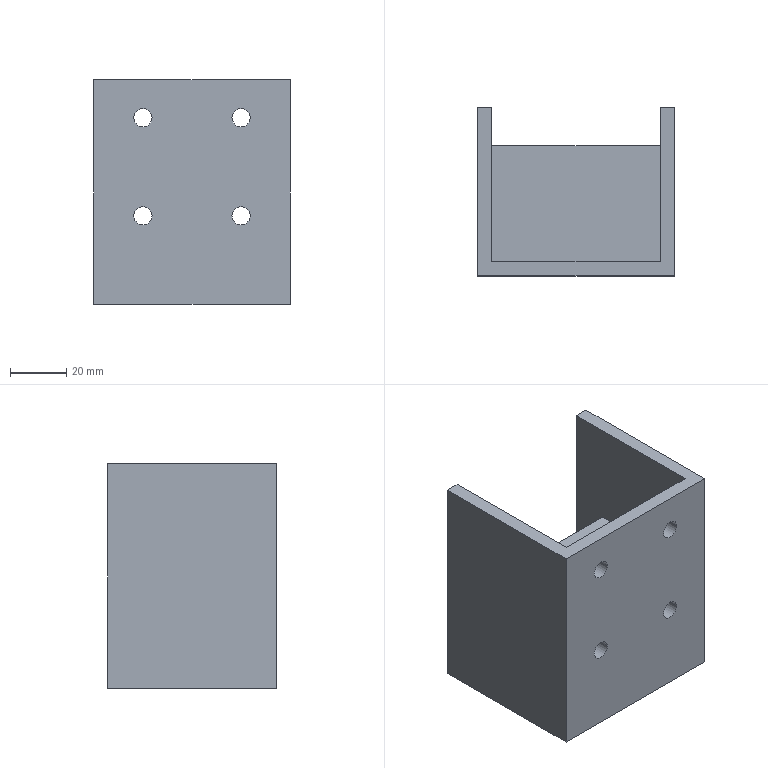Part | SolidWorks | features Cut 1, Extrusion 1, ICE 1 | 1 solid | 22 faces | box 70 x 60 x 80 mm | volume 83779 mm3 | plane 14 | cylinder 8 | commonest cylinder face diameters 6.5 x8
STEP:
#1=CARTESIAN_POINT('',(-20.75,-25.,26.5));
#2=VERTEX_POINT('',#1);
#3=CARTESIAN_POINT('',(-14.25,-25.,26.5));
#4=VERTEX_POINT('',#3);
#5=CARTESIAN_POINT('',(-17.5,-25.,26.5));
#6=DIRECTION('',(0.,-1.,0.));
#7=DIRECTION('',(0.,0.,-1.));
#8=AXIS2_PLACEMENT_3D('',#5,#6,#7);
#9=CIRCLE('',#8,3.25);
#10=EDGE_CURVE('',#2,#4,#9,.T.);
#11=ORIENTED_EDGE('',*,*,#10,.F.);
#12=CARTESIAN_POINT('',(-20.75,-30.,26.5));
#13=VERTEX_POINT('',#12);
#14=CARTESIAN_POINT('',(-20.75,-20.,26.5));
#15=DIRECTION('',(0.,-1.,0.));
#16=VECTOR('',#15,1000.);
#17=LINE('',#14,#16);
#18=EDGE_CURVE('',#2,#13,#17,.T.);
#19=ORIENTED_EDGE('',*,*,#18,.T.);
#20=CARTESIAN_POINT('',(-14.25,-30.,26.5));
#21=VERTEX_POINT('',#20);
#22=CARTESIAN_POINT('',(-17.5,-30.,26.5));
#23=DIRECTION('',(0.,-1.,0.));
#24=DIRECTION('',(1.,0.,0.));
#25=AXIS2_PLACEMENT_3D('',#22,#23,#24);
#26=CIRCLE('',#25,3.25);
#27=EDGE_CURVE('',#13,#21,#26,.T.);
#28=ORIENTED_EDGE('',*,*,#27,.T.);
#29=CARTESIAN_POINT('',(-14.25,-20.,26.5));
#30=DIRECTION('',(0.,-1.,0.));
#31=VECTOR('',#30,1000.);
#32=LINE('',#29,#31);
#33=EDGE_CURVE('',#4,#21,#32,.T.);
#34=ORIENTED_EDGE('',*,*,#33,.F.);
#35=EDGE_LOOP('',(#11,#19,#28,#34));
#36=FACE_OUTER_BOUND('',#35,.T.);
#37=CARTESIAN_POINT('',(-17.5,-20.,26.5));
#38=DIRECTION('',(0.,-1.,0.));
#39=DIRECTION('',(1.,0.,0.));
#40=AXIS2_PLACEMENT_3D('',#37,#38,#39);
#41=CYLINDRICAL_SURFACE('',#40,3.25);
#42=ADVANCED_FACE('',(#36),#41,.F.);
#43=CARTESIAN_POINT('',(-20.75,-25.,-8.5));
#44=VERTEX_POINT('',#43);
#45=CARTESIAN_POINT('',(-14.25,-25.,-8.5));
#46=VERTEX_POINT('',#45);
#47=CARTESIAN_POINT('',(-17.5,-25.,-8.5));
#48=DIRECTION('',(0.,-1.,0.));
#49=DIRECTION('',(0.,0.,-1.));
#50=AXIS2_PLACEMENT_3D('',#47,#48,#49);
#51=CIRCLE('',#50,3.25);
#52=EDGE_CURVE('',#44,#46,#51,.T.);
#53=ORIENTED_EDGE('',*,*,#52,.F.);
#54=CARTESIAN_POINT('',(-20.75,-30.,-8.5));
#55=VERTEX_POINT('',#54);
#56=CARTESIAN_POINT('',(-20.75,-20.,-8.5));
#57=DIRECTION('',(0.,-1.,0.));
#58=VECTOR('',#57,1000.);
#59=LINE('',#56,#58);
#60=EDGE_CURVE('',#44,#55,#59,.T.);
#61=ORIENTED_EDGE('',*,*,#60,.T.);
#62=CARTESIAN_POINT('',(-14.25,-30.,-8.5));
#63=VERTEX_POINT('',#62);
#64=CARTESIAN_POINT('',(-17.5,-30.,-8.5));
#65=DIRECTION('',(0.,-1.,0.));
#66=DIRECTION('',(1.,0.,0.));
#67=AXIS2_PLACEMENT_3D('',#64,#65,#66);
#68=CIRCLE('',#67,3.25);
#69=EDGE_CURVE('',#55,#63,#68,.T.);
#70=ORIENTED_EDGE('',*,*,#69,.T.);
#71=CARTESIAN_POINT('',(-14.25,-20.,-8.5));
#72=DIRECTION('',(0.,-1.,0.));
#73=VECTOR('',#72,1000.);
#74=LINE('',#71,#73);
#75=EDGE_CURVE('',#46,#63,#74,.T.);
#76=ORIENTED_EDGE('',*,*,#75,.F.);
#77=EDGE_LOOP('',(#53,#61,#70,#76));
#78=FACE_OUTER_BOUND('',#77,.T.);
#79=CARTESIAN_POINT('',(-17.5,-20.,-8.5));
#80=DIRECTION('',(0.,-1.,0.));
#81=DIRECTION('',(1.,0.,0.));
#82=AXIS2_PLACEMENT_3D('',#79,#80,#81);
#83=CYLINDRICAL_SURFACE('',#82,3.25);
#84=ADVANCED_FACE('',(#78),#83,.F.);
#85=CARTESIAN_POINT('',(14.25,-25.,-8.5));
#86=VERTEX_POINT('',#85);
#87=CARTESIAN_POINT('',(20.75,-25.,-8.5));
#88=VERTEX_POINT('',#87);
#89=CARTESIAN_POINT('',(17.5,-25.,-8.5));
#90=DIRECTION('',(0.,-1.,0.));
#91=DIRECTION('',(0.,0.,-1.));
#92=AXIS2_PLACEMENT_3D('',#89,#90,#91);
#93=CIRCLE('',#92,3.25);
#94=EDGE_CURVE('',#86,#88,#93,.T.);
#95=ORIENTED_EDGE('',*,*,#94,.F.);
#96=CARTESIAN_POINT('',(14.25,-30.,-8.5));
#97=VERTEX_POINT('',#96);
#98=CARTESIAN_POINT('',(14.25,-20.,-8.5));
#99=DIRECTION('',(0.,-1.,0.));
#100=VECTOR('',#99,1000.);
#101=LINE('',#98,#100);
#102=EDGE_CURVE('',#86,#97,#101,.T.);
#103=ORIENTED_EDGE('',*,*,#102,.T.);
#104=CARTESIAN_POINT('',(20.75,-30.,-8.5));
#105=VERTEX_POINT('',#104);
#106=CARTESIAN_POINT('',(17.5,-30.,-8.5));
#107=DIRECTION('',(0.,-1.,0.));
#108=DIRECTION('',(1.,0.,0.));
#109=AXIS2_PLACEMENT_3D('',#106,#107,#108);
#110=CIRCLE('',#109,3.25);
#111=EDGE_CURVE('',#97,#105,#110,.T.);
#112=ORIENTED_EDGE('',*,*,#111,.T.);
#113=CARTESIAN_POINT('',(20.75,-20.,-8.5));
#114=DIRECTION('',(0.,-1.,0.));
#115=VECTOR('',#114,1000.);
#116=LINE('',#113,#115);
#117=EDGE_CURVE('',#88,#105,#116,.T.);
#118=ORIENTED_EDGE('',*,*,#117,.F.);
#119=EDGE_LOOP('',(#95,#103,#112,#118));
#120=FACE_OUTER_BOUND('',#119,.T.);
#121=CARTESIAN_POINT('',(17.5,-20.,-8.5));
#122=DIRECTION('',(0.,-1.,0.));
#123=DIRECTION('',(1.,0.,0.));
#124=AXIS2_PLACEMENT_3D('',#121,#122,#123);
#125=CYLINDRICAL_SURFACE('',#124,3.25);
#126=ADVANCED_FACE('',(#120),#125,.F.);
#127=CARTESIAN_POINT('',(14.25,-25.,26.5));
#128=VERTEX_POINT('',#127);
#129=CARTESIAN_POINT('',(20.75,-25.,26.5));
#130=VERTEX_POINT('',#129);
#131=CARTESIAN_POINT('',(17.5,-25.,26.5));
#132=DIRECTION('',(0.,-1.,0.));
#133=DIRECTION('',(0.,0.,-1.));
#134=AXIS2_PLACEMENT_3D('',#131,#132,#133);
#135=CIRCLE('',#134,3.25);
#136=EDGE_CURVE('',#128,#130,#135,.T.);
#137=ORIENTED_EDGE('',*,*,#136,.F.);
#138=CARTESIAN_POINT('',(14.25,-30.,26.5));
#139=VERTEX_POINT('',#138);
#140=CARTESIAN_POINT('',(14.25,-20.,26.5));
#141=DIRECTION('',(0.,-1.,0.));
#142=VECTOR('',#141,1000.);
#143=LINE('',#140,#142);
#144=EDGE_CURVE('',#128,#139,#143,.T.);
#145=ORIENTED_EDGE('',*,*,#144,.T.);
#146=CARTESIAN_POINT('',(20.75,-30.,26.5));
#147=VERTEX_POINT('',#146);
#148=CARTESIAN_POINT('',(17.5,-30.,26.5));
#149=DIRECTION('',(0.,-1.,0.));
#150=DIRECTION('',(1.,0.,0.));
#151=AXIS2_PLACEMENT_3D('',#148,#149,#150);
#152=CIRCLE('',#151,3.25);
#153=EDGE_CURVE('',#139,#147,#152,.T.);
#154=ORIENTED_EDGE('',*,*,#153,.T.);
#155=CARTESIAN_POINT('',(20.75,-20.,26.5));
#156=DIRECTION('',(0.,-1.,0.));
#157=VECTOR('',#156,1000.);
#158=LINE('',#155,#157);
#159=EDGE_CURVE('',#130,#147,#158,.T.);
#160=ORIENTED_EDGE('',*,*,#159,.F.);
#161=EDGE_LOOP('',(#137,#145,#154,#160));
#162=FACE_OUTER_BOUND('',#161,.T.);
#163=CARTESIAN_POINT('',(17.5,-20.,26.5));
#164=DIRECTION('',(0.,-1.,0.));
#165=DIRECTION('',(1.,0.,0.));
#166=AXIS2_PLACEMENT_3D('',#163,#164,#165);
#167=CYLINDRICAL_SURFACE('',#166,3.25);
#168=ADVANCED_FACE('',(#162),#167,.F.);
#169=CARTESIAN_POINT('',(30.,-25.,2.5));
#170=VERTEX_POINT('',#169);
#171=CARTESIAN_POINT('',(30.,16.476,2.5));
#172=VERTEX_POINT('',#171);
#173=CARTESIAN_POINT('',(30.,-25.,2.5));
#174=DIRECTION('',(0.,1.,0.));
#175=VECTOR('',#174,1000.);
#176=LINE('',#173,#175);
#177=EDGE_CURVE('',#170,#172,#176,.T.);
#178=ORIENTED_EDGE('',*,*,#177,.F.);
#179=CARTESIAN_POINT('',(30.,-25.,40.));
#180=VERTEX_POINT('',#179);
#181=CARTESIAN_POINT('',(30.,-25.,40.));
#182=DIRECTION('',(0.,0.,-1.));
#183=VECTOR('',#182,1000.);
#184=LINE('',#181,#183);
#185=EDGE_CURVE('',#180,#170,#184,.T.);
#186=ORIENTED_EDGE('',*,*,#185,.F.);
#187=CARTESIAN_POINT('',(30.,30.,40.));
#188=VERTEX_POINT('',#187);
#189=CARTESIAN_POINT('',(30.,-25.,40.));
#190=DIRECTION('',(0.,-1.,0.));
#191=VECTOR('',#190,1000.);
#192=LINE('',#189,#191);
#193=EDGE_CURVE('',#188,#180,#192,.T.);
#194=ORIENTED_EDGE('',*,*,#193,.F.);
#195=CARTESIAN_POINT('',(30.,30.,-40.));
#196=VERTEX_POINT('',#195);
#197=CARTESIAN_POINT('',(30.,30.,40.));
#198=DIRECTION('',(0.,0.,-1.));
#199=VECTOR('',#198,1000.);
#200=LINE('',#197,#199);
#201=EDGE_CURVE('',#188,#196,#200,.T.);
#202=ORIENTED_EDGE('',*,*,#201,.T.);
#203=CARTESIAN_POINT('',(30.,-25.,-40.));
#204=VERTEX_POINT('',#203);
#205=CARTESIAN_POINT('',(30.,-25.,-40.));
#206=DIRECTION('',(0.,-1.,0.));
#207=VECTOR('',#206,1000.);
#208=LINE('',#205,#207);
#209=EDGE_CURVE('',#196,#204,#208,.T.);
#210=ORIENTED_EDGE('',*,*,#209,.T.);
#211=CARTESIAN_POINT('',(30.,-25.,-2.5));
#212=VERTEX_POINT('',#211);
#213=CARTESIAN_POINT('',(30.,-25.,40.));
#214=DIRECTION('',(0.,0.,-1.));
#215=VECTOR('',#214,1000.);
#216=LINE('',#213,#215);
#217=EDGE_CURVE('',#212,#204,#216,.T.);
#218=ORIENTED_EDGE('',*,*,#217,.F.);
#219=CARTESIAN_POINT('',(30.,16.476,-2.5));
#220=VERTEX_POINT('',#219);
#221=CARTESIAN_POINT('',(30.,-25.,-2.5));
#222=DIRECTION('',(0.,1.,0.));
#223=VECTOR('',#222,1000.);
#224=LINE('',#221,#223);
#225=EDGE_CURVE('',#212,#220,#224,.T.);
#226=ORIENTED_EDGE('',*,*,#225,.T.);
#227=CARTESIAN_POINT('',(30.,16.476,2.5));
#228=DIRECTION('',(0.,0.,-1.));
#229=VECTOR('',#228,1000.);
#230=LINE('',#227,#229);
#231=EDGE_CURVE('',#172,#220,#230,.T.);
#232=ORIENTED_EDGE('',*,*,#231,.F.);
#233=EDGE_LOOP('',(#178,#186,#194,#202,#210,#218,#226,#232));
#234=FACE_OUTER_BOUND('',#233,.T.);
#235=CARTESIAN_POINT('',(30.,-25.,40.));
#236=DIRECTION('',(1.,0.,0.));
#237=DIRECTION('',(0.,1.,0.));
#238=AXIS2_PLACEMENT_3D('',#235,#236,#237);
#239=PLANE('',#238);
#240=ADVANCED_FACE('',(#234),#239,.F.);
#241=CARTESIAN_POINT('',(-17.5,-25.,26.5));
#242=DIRECTION('',(0.,-1.,0.));
#243=DIRECTION('',(0.,0.,-1.));
#244=AXIS2_PLACEMENT_3D('',#241,#242,#243);
#245=CIRCLE('',#244,3.25);
#246=EDGE_CURVE('',#4,#2,#245,.T.);
#247=ORIENTED_EDGE('',*,*,#246,.T.);
#248=ORIENTED_EDGE('',*,*,#10,.T.);
#249=EDGE_LOOP('',(#247,#248));
#250=FACE_BOUND('',#249,.T.);
#251=CARTESIAN_POINT('',(17.5,-25.,26.5));
#252=DIRECTION('',(0.,-1.,0.));
#253=DIRECTION('',(0.,0.,-1.));
#254=AXIS2_PLACEMENT_3D('',#251,#252,#253);
#255=CIRCLE('',#254,3.25);
#256=EDGE_CURVE('',#130,#128,#255,.T.);
#257=ORIENTED_EDGE('',*,*,#256,.T.);
#258=ORIENTED_EDGE('',*,*,#136,.T.);
#259=EDGE_LOOP('',(#257,#258));
#260=FACE_BOUND('',#259,.T.);
#261=CARTESIAN_POINT('',(-30.,-25.,2.5));
#262=VERTEX_POINT('',#261);
#263=CARTESIAN_POINT('',(-30.,-25.,2.5));
#264=DIRECTION('',(1.,0.,0.));
#265=VECTOR('',#264,1000.);
#266=LINE('',#263,#265);
#267=EDGE_CURVE('',#262,#170,#266,.T.);
#268=ORIENTED_EDGE('',*,*,#267,.F.);
#269=CARTESIAN_POINT('',(-30.,-25.,40.));
#270=VERTEX_POINT('',#269);
#271=CARTESIAN_POINT('',(-30.,-25.,40.));
#272=DIRECTION('',(0.,0.,-1.));
#273=VECTOR('',#272,1000.);
#274=LINE('',#271,#273);
#275=EDGE_CURVE('',#270,#262,#274,.T.);
#276=ORIENTED_EDGE('',*,*,#275,.F.);
#277=CARTESIAN_POINT('',(-30.,-25.,40.));
#278=DIRECTION('',(-1.,0.,0.));
#279=VECTOR('',#278,1000.);
#280=LINE('',#277,#279);
#281=EDGE_CURVE('',#180,#270,#280,.T.);
#282=ORIENTED_EDGE('',*,*,#281,.F.);
#283=ORIENTED_EDGE('',*,*,#185,.T.);
#284=EDGE_LOOP('',(#268,#276,#282,#283));
#285=FACE_OUTER_BOUND('',#284,.T.);
#286=CARTESIAN_POINT('',(-30.,-25.,40.));
#287=DIRECTION('',(0.,-1.,0.));
#288=DIRECTION('',(0.,0.,-1.));
#289=AXIS2_PLACEMENT_3D('',#286,#287,#288);
#290=PLANE('',#289);
#291=ADVANCED_FACE('',(#250,#260,#285),#290,.F.);
#292=CARTESIAN_POINT('',(-30.,16.476,2.5));
#293=VERTEX_POINT('',#292);
#294=CARTESIAN_POINT('',(-30.,-25.,2.5));
#295=DIRECTION('',(0.,-1.,0.));
#296=VECTOR('',#295,1000.);
#297=LINE('',#294,#296);
#298=EDGE_CURVE('',#293,#262,#297,.T.);
#299=ORIENTED_EDGE('',*,*,#298,.F.);
#300=CARTESIAN_POINT('',(-30.,16.476,-2.5));
#301=VERTEX_POINT('',#300);
#302=CARTESIAN_POINT('',(-30.,16.476,2.5));
#303=DIRECTION('',(0.,0.,-1.));
#304=VECTOR('',#303,1000.);
#305=LINE('',#302,#304);
#306=EDGE_CURVE('',#293,#301,#305,.T.);
#307=ORIENTED_EDGE('',*,*,#306,.T.);
#308=CARTESIAN_POINT('',(-30.,-25.,-2.5));
#309=VERTEX_POINT('',#308);
#310=CARTESIAN_POINT('',(-30.,-25.,-2.5));
#311=DIRECTION('',(0.,-1.,0.));
#312=VECTOR('',#311,1000.);
#313=LINE('',#310,#312);
#314=EDGE_CURVE('',#301,#309,#313,.T.);
#315=ORIENTED_EDGE('',*,*,#314,.T.);
#316=CARTESIAN_POINT('',(-30.,-25.,-40.));
#317=VERTEX_POINT('',#316);
#318=CARTESIAN_POINT('',(-30.,-25.,40.));
#319=DIRECTION('',(0.,0.,-1.));
#320=VECTOR('',#319,1000.);
#321=LINE('',#318,#320);
#322=EDGE_CURVE('',#309,#317,#321,.T.);
#323=ORIENTED_EDGE('',*,*,#322,.T.);
#324=CARTESIAN_POINT('',(-30.,30.,-40.));
#325=VERTEX_POINT('',#324);
#326=CARTESIAN_POINT('',(-30.,30.,-40.));
#327=DIRECTION('',(0.,1.,0.));
#328=VECTOR('',#327,1000.);
#329=LINE('',#326,#328);
#330=EDGE_CURVE('',#317,#325,#329,.T.);
#331=ORIENTED_EDGE('',*,*,#330,.T.);
#332=CARTESIAN_POINT('',(-30.,30.,40.));
#333=VERTEX_POINT('',#332);
#334=CARTESIAN_POINT('',(-30.,30.,40.));
#335=DIRECTION('',(0.,0.,-1.));
#336=VECTOR('',#335,1000.);
#337=LINE('',#334,#336);
#338=EDGE_CURVE('',#333,#325,#337,.T.);
#339=ORIENTED_EDGE('',*,*,#338,.F.);
#340=CARTESIAN_POINT('',(-30.,30.,40.));
#341=DIRECTION('',(0.,1.,0.));
#342=VECTOR('',#341,1000.);
#343=LINE('',#340,#342);
#344=EDGE_CURVE('',#270,#333,#343,.T.);
#345=ORIENTED_EDGE('',*,*,#344,.F.);
#346=ORIENTED_EDGE('',*,*,#275,.T.);
#347=EDGE_LOOP('',(#299,#307,#315,#323,#331,#339,#345,#346));
#348=FACE_OUTER_BOUND('',#347,.T.);
#349=CARTESIAN_POINT('',(-30.,30.,40.));
#350=DIRECTION('',(-1.,0.,0.));
#351=DIRECTION('',(0.,-1.,0.));
#352=AXIS2_PLACEMENT_3D('',#349,#350,#351);
#353=PLANE('',#352);
#354=ADVANCED_FACE('',(#348),#353,.F.);
#355=CARTESIAN_POINT('',(-35.,30.,-40.));
#356=VERTEX_POINT('',#355);
#357=CARTESIAN_POINT('',(-30.,30.,-40.));
#358=DIRECTION('',(-1.,0.,0.));
#359=VECTOR('',#358,1000.);
#360=LINE('',#357,#359);
#361=EDGE_CURVE('',#325,#356,#360,.T.);
#362=ORIENTED_EDGE('',*,*,#361,.T.);
#363=CARTESIAN_POINT('',(-35.,30.,40.));
#364=VERTEX_POINT('',#363);
#365=CARTESIAN_POINT('',(-35.,30.,40.));
#366=DIRECTION('',(0.,0.,-1.));
#367=VECTOR('',#366,1000.);
#368=LINE('',#365,#367);
#369=EDGE_CURVE('',#364,#356,#368,.T.);
#370=ORIENTED_EDGE('',*,*,#369,.F.);
#371=CARTESIAN_POINT('',(-30.,30.,40.));
#372=DIRECTION('',(-1.,0.,0.));
#373=VECTOR('',#372,1000.);
#374=LINE('',#371,#373);
#375=EDGE_CURVE('',#333,#364,#374,.T.);
#376=ORIENTED_EDGE('',*,*,#375,.F.);
#377=ORIENTED_EDGE('',*,*,#338,.T.);
#378=EDGE_LOOP('',(#362,#370,#376,#377));
#379=FACE_OUTER_BOUND('',#378,.T.);
#380=CARTESIAN_POINT('',(-30.,30.,40.));
#381=DIRECTION('',(0.,-1.,0.));
#382=DIRECTION('',(0.,0.,-1.));
#383=AXIS2_PLACEMENT_3D('',#380,#381,#382);
#384=PLANE('',#383);
#385=ADVANCED_FACE('',(#379),#384,.F.);
#386=CARTESIAN_POINT('',(-35.,-30.,-40.));
#387=VERTEX_POINT('',#386);
#388=CARTESIAN_POINT('',(-35.,-30.,-40.));
#389=DIRECTION('',(0.,-1.,0.));
#390=VECTOR('',#389,1000.);
#391=LINE('',#388,#390);
#392=EDGE_CURVE('',#356,#387,#391,.T.);
#393=ORIENTED_EDGE('',*,*,#392,.T.);
#394=CARTESIAN_POINT('',(-35.,-30.,40.));
#395=VERTEX_POINT('',#394);
#396=CARTESIAN_POINT('',(-35.,-30.,40.));
#397=DIRECTION('',(0.,0.,-1.));
#398=VECTOR('',#397,1000.);
#399=LINE('',#396,#398);
#400=EDGE_CURVE('',#395,#387,#399,.T.);
#401=ORIENTED_EDGE('',*,*,#400,.F.);
#402=CARTESIAN_POINT('',(-35.,-30.,40.));
#403=DIRECTION('',(0.,-1.,0.));
#404=VECTOR('',#403,1000.);
#405=LINE('',#402,#404);
#406=EDGE_CURVE('',#364,#395,#405,.T.);
#407=ORIENTED_EDGE('',*,*,#406,.F.);
#408=ORIENTED_EDGE('',*,*,#369,.T.);
#409=EDGE_LOOP('',(#393,#401,#407,#408));
#410=FACE_OUTER_BOUND('',#409,.T.);
#411=CARTESIAN_POINT('',(-35.,-30.,40.));
#412=DIRECTION('',(1.,0.,0.));
#413=DIRECTION('',(0.,0.,-1.));
#414=AXIS2_PLACEMENT_3D('',#411,#412,#413);
#415=PLANE('',#414);
#416=ADVANCED_FACE('',(#410),#415,.F.);
#417=CARTESIAN_POINT('',(-17.5,-30.,26.5));
#418=DIRECTION('',(0.,-1.,0.));
#419=DIRECTION('',(1.,0.,0.));
#420=AXIS2_PLACEMENT_3D('',#417,#418,#419);
#421=CIRCLE('',#420,3.25);
#422=EDGE_CURVE('',#21,#13,#421,.T.);
#423=ORIENTED_EDGE('',*,*,#422,.F.);
#424=ORIENTED_EDGE('',*,*,#27,.F.);
#425=EDGE_LOOP('',(#423,#424));
#426=FACE_BOUND('',#425,.T.);
#427=CARTESIAN_POINT('',(-17.5,-30.,-8.5));
#428=DIRECTION('',(0.,-1.,0.));
#429=DIRECTION('',(1.,0.,0.));
#430=AXIS2_PLACEMENT_3D('',#427,#428,#429);
#431=CIRCLE('',#430,3.25);
#432=EDGE_CURVE('',#63,#55,#431,.T.);
#433=ORIENTED_EDGE('',*,*,#432,.F.);
#434=ORIENTED_EDGE('',*,*,#69,.F.);
#435=EDGE_LOOP('',(#433,#434));
#436=FACE_BOUND('',#435,.T.);
#437=CARTESIAN_POINT('',(17.5,-30.,-8.5));
#438=DIRECTION('',(0.,-1.,0.));
#439=DIRECTION('',(1.,0.,0.));
#440=AXIS2_PLACEMENT_3D('',#437,#438,#439);
#441=CIRCLE('',#440,3.25);
#442=EDGE_CURVE('',#105,#97,#441,.T.);
#443=ORIENTED_EDGE('',*,*,#442,.F.);
#444=ORIENTED_EDGE('',*,*,#111,.F.);
#445=EDGE_LOOP('',(#443,#444));
#446=FACE_BOUND('',#445,.T.);
#447=CARTESIAN_POINT('',(17.5,-30.,26.5));
#448=DIRECTION('',(0.,-1.,0.));
#449=DIRECTION('',(1.,0.,0.));
#450=AXIS2_PLACEMENT_3D('',#447,#448,#449);
#451=CIRCLE('',#450,3.25);
#452=EDGE_CURVE('',#147,#139,#451,.T.);
#453=ORIENTED_EDGE('',*,*,#452,.F.);
#454=ORIENTED_EDGE('',*,*,#153,.F.);
#455=EDGE_LOOP('',(#453,#454));
#456=FACE_BOUND('',#455,.T.);
#457=CARTESIAN_POINT('',(35.,-30.,-40.));
#458=VERTEX_POINT('',#457);
#459=CARTESIAN_POINT('',(35.,-30.,-40.));
#460=DIRECTION('',(1.,0.,0.));
#461=VECTOR('',#460,1000.);
#462=LINE('',#459,#461);
#463=EDGE_CURVE('',#387,#458,#462,.T.);
#464=ORIENTED_EDGE('',*,*,#463,.T.);
#465=CARTESIAN_POINT('',(35.,-30.,40.));
#466=VERTEX_POINT('',#465);
#467=CARTESIAN_POINT('',(35.,-30.,40.));
#468=DIRECTION('',(0.,0.,-1.));
#469=VECTOR('',#468,1000.);
#470=LINE('',#467,#469);
#471=EDGE_CURVE('',#466,#458,#470,.T.);
#472=ORIENTED_EDGE('',*,*,#471,.F.);
#473=CARTESIAN_POINT('',(35.,-30.,40.));
#474=DIRECTION('',(1.,0.,0.));
#475=VECTOR('',#474,1000.);
#476=LINE('',#473,#475);
#477=EDGE_CURVE('',#395,#466,#476,.T.);
#478=ORIENTED_EDGE('',*,*,#477,.F.);
#479=ORIENTED_EDGE('',*,*,#400,.T.);
#480=EDGE_LOOP('',(#464,#472,#478,#479));
#481=FACE_OUTER_BOUND('',#480,.T.);
#482=CARTESIAN_POINT('',(35.,-30.,40.));
#483=DIRECTION('',(0.,1.,0.));
#484=DIRECTION('',(-1.,0.,0.));
#485=AXIS2_PLACEMENT_3D('',#482,#483,#484);
#486=PLANE('',#485);
#487=ADVANCED_FACE('',(#426,#436,#446,#456,#481),#486,.F.);
#488=CARTESIAN_POINT('',(35.,30.,-40.));
#489=VERTEX_POINT('',#488);
#490=CARTESIAN_POINT('',(35.,-30.,-40.));
#491=DIRECTION('',(0.,1.,0.));
#492=VECTOR('',#491,1000.);
#493=LINE('',#490,#492);
#494=EDGE_CURVE('',#458,#489,#493,.T.);
#495=ORIENTED_EDGE('',*,*,#494,.T.);
#496=CARTESIAN_POINT('',(35.,30.,40.));
#497=VERTEX_POINT('',#496);
#498=CARTESIAN_POINT('',(35.,30.,40.));
#499=DIRECTION('',(0.,0.,-1.));
#500=VECTOR('',#499,1000.);
#501=LINE('',#498,#500);
#502=EDGE_CURVE('',#497,#489,#501,.T.);
#503=ORIENTED_EDGE('',*,*,#502,.F.);
#504=CARTESIAN_POINT('',(35.,-30.,40.));
#505=DIRECTION('',(0.,1.,0.));
#506=VECTOR('',#505,1000.);
#507=LINE('',#504,#506);
#508=EDGE_CURVE('',#466,#497,#507,.T.);
#509=ORIENTED_EDGE('',*,*,#508,.F.);
#510=ORIENTED_EDGE('',*,*,#471,.T.);
#511=EDGE_LOOP('',(#495,#503,#509,#510));
#512=FACE_OUTER_BOUND('',#511,.T.);
#513=CARTESIAN_POINT('',(35.,-30.,40.));
#514=DIRECTION('',(-1.,0.,0.));
#515=DIRECTION('',(0.,0.,1.));
#516=AXIS2_PLACEMENT_3D('',#513,#514,#515);
#517=PLANE('',#516);
#518=ADVANCED_FACE('',(#512),#517,.F.);
#519=CARTESIAN_POINT('',(35.,30.,-40.));
#520=DIRECTION('',(-1.,0.,0.));
#521=VECTOR('',#520,1000.);
#522=LINE('',#519,#521);
#523=EDGE_CURVE('',#489,#196,#522,.T.);
#524=ORIENTED_EDGE('',*,*,#523,.T.);
#525=ORIENTED_EDGE('',*,*,#201,.F.);
#526=CARTESIAN_POINT('',(35.,30.,40.));
#527=DIRECTION('',(-1.,0.,0.));
#528=VECTOR('',#527,1000.);
#529=LINE('',#526,#528);
#530=EDGE_CURVE('',#497,#188,#529,.T.);
#531=ORIENTED_EDGE('',*,*,#530,.F.);
#532=ORIENTED_EDGE('',*,*,#502,.T.);
#533=EDGE_LOOP('',(#524,#525,#531,#532));
#534=FACE_OUTER_BOUND('',#533,.T.);
#535=CARTESIAN_POINT('',(35.,30.,40.));
#536=DIRECTION('',(0.,-1.,0.));
#537=DIRECTION('',(1.,0.,0.));
#538=AXIS2_PLACEMENT_3D('',#535,#536,#537);
#539=PLANE('',#538);
#540=ADVANCED_FACE('',(#534),#539,.F.);
#541=CARTESIAN_POINT('',(-17.5,-25.,-8.5));
#542=DIRECTION('',(0.,-1.,0.));
#543=DIRECTION('',(0.,0.,-1.));
#544=AXIS2_PLACEMENT_3D('',#541,#542,#543);
#545=CIRCLE('',#544,3.25);
#546=EDGE_CURVE('',#46,#44,#545,.T.);
#547=ORIENTED_EDGE('',*,*,#546,.T.);
#548=ORIENTED_EDGE('',*,*,#52,.T.);
#549=EDGE_LOOP('',(#547,#548));
#550=FACE_BOUND('',#549,.T.);
#551=CARTESIAN_POINT('',(17.5,-25.,-8.5));
#552=DIRECTION('',(0.,-1.,0.));
#553=DIRECTION('',(0.,0.,-1.));
#554=AXIS2_PLACEMENT_3D('',#551,#552,#553);
#555=CIRCLE('',#554,3.25);
#556=EDGE_CURVE('',#88,#86,#555,.T.);
#557=ORIENTED_EDGE('',*,*,#556,.T.);
#558=ORIENTED_EDGE('',*,*,#94,.T.);
#559=EDGE_LOOP('',(#557,#558));
#560=FACE_BOUND('',#559,.T.);
#561=ORIENTED_EDGE('',*,*,#322,.F.);
#562=CARTESIAN_POINT('',(-30.,-25.,-2.5));
#563=DIRECTION('',(1.,0.,0.));
#564=VECTOR('',#563,1000.);
#565=LINE('',#562,#564);
#566=EDGE_CURVE('',#309,#212,#565,.T.);
#567=ORIENTED_EDGE('',*,*,#566,.T.);
#568=ORIENTED_EDGE('',*,*,#217,.T.);
#569=CARTESIAN_POINT('',(-30.,-25.,-40.));
#570=DIRECTION('',(-1.,0.,0.));
#571=VECTOR('',#570,1000.);
#572=LINE('',#569,#571);
#573=EDGE_CURVE('',#204,#317,#572,.T.);
#574=ORIENTED_EDGE('',*,*,#573,.T.);
#575=EDGE_LOOP('',(#561,#567,#568,#574));
#576=FACE_OUTER_BOUND('',#575,.T.);
#577=CARTESIAN_POINT('',(-30.,-25.,40.));
#578=DIRECTION('',(0.,-1.,0.));
#579=DIRECTION('',(0.,0.,-1.));
#580=AXIS2_PLACEMENT_3D('',#577,#578,#579);
#581=PLANE('',#580);
#582=ADVANCED_FACE('',(#550,#560,#576),#581,.F.);
#583=ORIENTED_EDGE('',*,*,#375,.T.);
#584=ORIENTED_EDGE('',*,*,#406,.T.);
#585=ORIENTED_EDGE('',*,*,#477,.T.);
#586=ORIENTED_EDGE('',*,*,#508,.T.);
#587=ORIENTED_EDGE('',*,*,#530,.T.);
#588=ORIENTED_EDGE('',*,*,#193,.T.);
#589=ORIENTED_EDGE('',*,*,#281,.T.);
#590=ORIENTED_EDGE('',*,*,#344,.T.);
#591=EDGE_LOOP('',(#583,#584,#585,#586,#587,#588,#589,#590));
#592=FACE_OUTER_BOUND('',#591,.T.);
#593=CARTESIAN_POINT('',(0.,0.,40.));
#594=DIRECTION('',(0.,0.,-1.));
#595=DIRECTION('',(-1.,0.,0.));
#596=AXIS2_PLACEMENT_3D('',#593,#594,#595);
#597=PLANE('',#596);
#598=ADVANCED_FACE('',(#592),#597,.F.);
#599=ORIENTED_EDGE('',*,*,#361,.F.);
#600=ORIENTED_EDGE('',*,*,#330,.F.);
#601=ORIENTED_EDGE('',*,*,#573,.F.);
#602=ORIENTED_EDGE('',*,*,#209,.F.);
#603=ORIENTED_EDGE('',*,*,#523,.F.);
#604=ORIENTED_EDGE('',*,*,#494,.F.);
#605=ORIENTED_EDGE('',*,*,#463,.F.);
#606=ORIENTED_EDGE('',*,*,#392,.F.);
#607=EDGE_LOOP('',(#599,#600,#601,#602,#603,#604,#605,#606));
#608=FACE_OUTER_BOUND('',#607,.T.);
#609=CARTESIAN_POINT('',(0.,0.,-40.));
#610=DIRECTION('',(0.,0.,-1.));
#611=DIRECTION('',(-1.,0.,0.));
#612=AXIS2_PLACEMENT_3D('',#609,#610,#611);
#613=PLANE('',#612);
#614=ADVANCED_FACE('',(#608),#613,.T.);
#615=CARTESIAN_POINT('',(-30.,16.476,-2.5));
#616=DIRECTION('',(-1.,0.,0.));
#617=VECTOR('',#616,1000.);
#618=LINE('',#615,#617);
#619=EDGE_CURVE('',#220,#301,#618,.T.);
#620=ORIENTED_EDGE('',*,*,#619,.T.);
#621=ORIENTED_EDGE('',*,*,#306,.F.);
#622=CARTESIAN_POINT('',(-30.,16.476,2.5));
#623=DIRECTION('',(-1.,0.,0.));
#624=VECTOR('',#623,1000.);
#625=LINE('',#622,#624);
#626=EDGE_CURVE('',#172,#293,#625,.T.);
#627=ORIENTED_EDGE('',*,*,#626,.F.);
#628=ORIENTED_EDGE('',*,*,#231,.T.);
#629=EDGE_LOOP('',(#620,#621,#627,#628));
#630=FACE_OUTER_BOUND('',#629,.T.);
#631=CARTESIAN_POINT('',(-30.,16.476,2.5));
#632=DIRECTION('',(0.,-1.,0.));
#633=DIRECTION('',(0.,0.,-1.));
#634=AXIS2_PLACEMENT_3D('',#631,#632,#633);
#635=PLANE('',#634);
#636=ADVANCED_FACE('',(#630),#635,.F.);
#637=ORIENTED_EDGE('',*,*,#298,.T.);
#638=ORIENTED_EDGE('',*,*,#267,.T.);
#639=ORIENTED_EDGE('',*,*,#177,.T.);
#640=ORIENTED_EDGE('',*,*,#626,.T.);
#641=EDGE_LOOP('',(#637,#638,#639,#640));
#642=FACE_OUTER_BOUND('',#641,.T.);
#643=CARTESIAN_POINT('',(0.,0.,2.5));
#644=DIRECTION('',(0.,0.,-1.));
#645=DIRECTION('',(-1.,0.,0.));
#646=AXIS2_PLACEMENT_3D('',#643,#644,#645);
#647=PLANE('',#646);
#648=ADVANCED_FACE('',(#642),#647,.F.);
#649=ORIENTED_EDGE('',*,*,#314,.F.);
#650=ORIENTED_EDGE('',*,*,#619,.F.);
#651=ORIENTED_EDGE('',*,*,#225,.F.);
#652=ORIENTED_EDGE('',*,*,#566,.F.);
#653=EDGE_LOOP('',(#649,#650,#651,#652));
#654=FACE_OUTER_BOUND('',#653,.T.);
#655=CARTESIAN_POINT('',(0.,0.,-2.5));
#656=DIRECTION('',(0.,0.,-1.));
#657=DIRECTION('',(-1.,0.,0.));
#658=AXIS2_PLACEMENT_3D('',#655,#656,#657);
#659=PLANE('',#658);
#660=ADVANCED_FACE('',(#654),#659,.T.);
#661=ORIENTED_EDGE('',*,*,#144,.F.);
#662=ORIENTED_EDGE('',*,*,#256,.F.);
#663=ORIENTED_EDGE('',*,*,#159,.T.);
#664=ORIENTED_EDGE('',*,*,#452,.T.);
#665=EDGE_LOOP('',(#661,#662,#663,#664));
#666=FACE_OUTER_BOUND('',#665,.T.);
#667=CARTESIAN_POINT('',(17.5,-20.,26.5));
#668=DIRECTION('',(0.,-1.,0.));
#669=DIRECTION('',(1.,0.,0.));
#670=AXIS2_PLACEMENT_3D('',#667,#668,#669);
#671=CYLINDRICAL_SURFACE('',#670,3.25);
#672=ADVANCED_FACE('',(#666),#671,.F.);
#673=ORIENTED_EDGE('',*,*,#102,.F.);
#674=ORIENTED_EDGE('',*,*,#556,.F.);
#675=ORIENTED_EDGE('',*,*,#117,.T.);
#676=ORIENTED_EDGE('',*,*,#442,.T.);
#677=EDGE_LOOP('',(#673,#674,#675,#676));
#678=FACE_OUTER_BOUND('',#677,.T.);
#679=CARTESIAN_POINT('',(17.5,-20.,-8.5));
#680=DIRECTION('',(0.,-1.,0.));
#681=DIRECTION('',(1.,0.,0.));
#682=AXIS2_PLACEMENT_3D('',#679,#680,#681);
#683=CYLINDRICAL_SURFACE('',#682,3.25);
#684=ADVANCED_FACE('',(#678),#683,.F.);
#685=ORIENTED_EDGE('',*,*,#60,.F.);
#686=ORIENTED_EDGE('',*,*,#546,.F.);
#687=ORIENTED_EDGE('',*,*,#75,.T.);
#688=ORIENTED_EDGE('',*,*,#432,.T.);
#689=EDGE_LOOP('',(#685,#686,#687,#688));
#690=FACE_OUTER_BOUND('',#689,.T.);
#691=CARTESIAN_POINT('',(-17.5,-20.,-8.5));
#692=DIRECTION('',(0.,-1.,0.));
#693=DIRECTION('',(1.,0.,0.));
#694=AXIS2_PLACEMENT_3D('',#691,#692,#693);
#695=CYLINDRICAL_SURFACE('',#694,3.25);
#696=ADVANCED_FACE('',(#690),#695,.F.);
#697=ORIENTED_EDGE('',*,*,#18,.F.);
#698=ORIENTED_EDGE('',*,*,#246,.F.);
#699=ORIENTED_EDGE('',*,*,#33,.T.);
#700=ORIENTED_EDGE('',*,*,#422,.T.);
#701=EDGE_LOOP('',(#697,#698,#699,#700));
#702=FACE_OUTER_BOUND('',#701,.T.);
#703=CARTESIAN_POINT('',(-17.5,-20.,26.5));
#704=DIRECTION('',(0.,-1.,0.));
#705=DIRECTION('',(1.,0.,0.));
#706=AXIS2_PLACEMENT_3D('',#703,#704,#705);
#707=CYLINDRICAL_SURFACE('',#706,3.25);
#708=ADVANCED_FACE('',(#702),#707,.F.);
#709=CLOSED_SHELL('',(#42,#84,#126,#168,#240,#291,#354,#385,#416,#487,#518,#540,#582,#598,#614,#636,#648,#660,#672,#684,#696,#708));
#710=MANIFOLD_SOLID_BREP('',#709);
#711=CARTESIAN_POINT('',(0.,0.,0.));
#712=DIRECTION('',(0.,0.,1.));
#713=DIRECTION('',(1.,0.,0.));
#714=AXIS2_PLACEMENT_3D('',#711,#712,#713);
#715=(LENGTH_UNIT()NAMED_UNIT(*)SI_UNIT(.MILLI.,.METRE.));
#716=UNCERTAINTY_MEASURE_WITH_UNIT(LENGTH_MEASURE(0.00001),#715,'','');
#717=(NAMED_UNIT(*)PLANE_ANGLE_UNIT()SI_UNIT($,.RADIAN.));
#718=(NAMED_UNIT(*)SI_UNIT($,.STERADIAN.)SOLID_ANGLE_UNIT());
#719=(GEOMETRIC_REPRESENTATION_CONTEXT(3)GLOBAL_UNCERTAINTY_ASSIGNED_CONTEXT((#716))GLOBAL_UNIT_ASSIGNED_CONTEXT((#715,#717,#718))REPRESENTATION_CONTEXT('',''));
#720=ADVANCED_BREP_SHAPE_REPRESENTATION('',(#710,#714),#719);